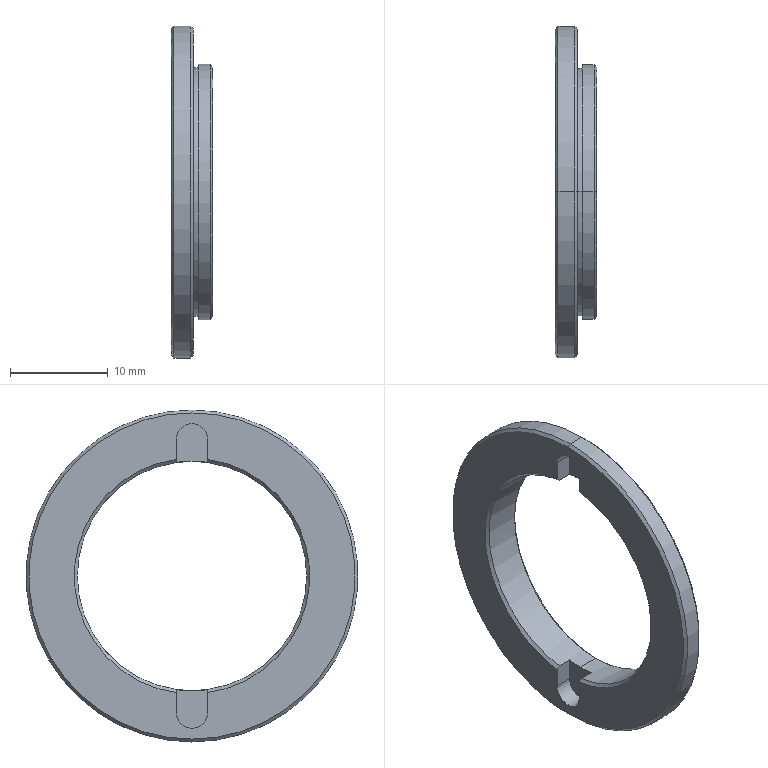Part | STEP file | CRM-1A-1-3-ZA.step-14.STEP.STEP-83.STEP | 1 solid | 31 faces | box 4.3 x 34 x 34 mm | volume 1225 mm3 | cylinder 11 | cone 10 | plane 10 | commonest cylinder face diameters 3.2 x3 23.5 x2 25.4 x2 26.2 x2 34 x2
STEP:
#1=CARTESIAN_POINT('',(1.8,0.,15.6));
#2=VERTEX_POINT('',#1);
#3=CARTESIAN_POINT('',(1.8,1.6,14.));
#4=VERTEX_POINT('',#3);
#5=CARTESIAN_POINT('',(1.8,0.,14.));
#6=DIRECTION('',(-1.,0.,0.));
#7=DIRECTION('',(0.,0.,-1.));
#8=AXIS2_PLACEMENT_3D('',#5,#6,#7);
#9=CIRCLE('',#8,1.6);
#10=EDGE_CURVE('',#2,#4,#9,.T.);
#11=ORIENTED_EDGE('',*,*,#10,.F.);
#12=CARTESIAN_POINT('',(0.,0.,15.6));
#13=VERTEX_POINT('',#12);
#14=CARTESIAN_POINT('',(1.8,0.,15.6));
#15=DIRECTION('',(-1.,0.,0.));
#16=VECTOR('',#15,1000.);
#17=LINE('',#14,#16);
#18=EDGE_CURVE('',#2,#13,#17,.T.);
#19=ORIENTED_EDGE('',*,*,#18,.T.);
#20=CARTESIAN_POINT('',(0.,1.6,14.));
#21=VERTEX_POINT('',#20);
#22=CARTESIAN_POINT('',(0.,0.,14.));
#23=DIRECTION('',(-1.,0.,0.));
#24=DIRECTION('',(0.,0.,-1.));
#25=AXIS2_PLACEMENT_3D('',#22,#23,#24);
#26=CIRCLE('',#25,1.6);
#27=EDGE_CURVE('',#13,#21,#26,.T.);
#28=ORIENTED_EDGE('',*,*,#27,.T.);
#29=CARTESIAN_POINT('',(1.8,1.6,14.));
#30=DIRECTION('',(-1.,0.,0.));
#31=VECTOR('',#30,1000.);
#32=LINE('',#29,#31);
#33=EDGE_CURVE('',#4,#21,#32,.T.);
#34=ORIENTED_EDGE('',*,*,#33,.F.);
#35=EDGE_LOOP('',(#11,#19,#28,#34));
#36=FACE_OUTER_BOUND('',#35,.T.);
#37=CARTESIAN_POINT('',(1.8,0.,14.));
#38=DIRECTION('',(-1.,0.,0.));
#39=DIRECTION('',(0.,0.,1.));
#40=AXIS2_PLACEMENT_3D('',#37,#38,#39);
#41=CYLINDRICAL_SURFACE('',#40,1.6);
#42=ADVANCED_FACE('',(#36),#41,.F.);
#43=CARTESIAN_POINT('',(4.3,0.,-12.8));
#44=VERTEX_POINT('',#43);
#45=CARTESIAN_POINT('',(4.3,0.,12.8));
#46=VERTEX_POINT('',#45);
#47=CARTESIAN_POINT('',(4.3,0.,0.));
#48=DIRECTION('',(1.,0.,0.));
#49=DIRECTION('',(0.,0.,1.));
#50=AXIS2_PLACEMENT_3D('',#47,#48,#49);
#51=CIRCLE('',#50,12.8);
#52=EDGE_CURVE('',#44,#46,#51,.T.);
#53=ORIENTED_EDGE('',*,*,#52,.F.);
#54=CARTESIAN_POINT('',(4.,0.,-13.1));
#55=VERTEX_POINT('',#54);
#56=CARTESIAN_POINT('',(4.,0.,-13.1));
#57=DIRECTION('',(-0.7071,0.,-0.7071));
#58=VECTOR('',#57,1000.);
#59=LINE('',#56,#58);
#60=EDGE_CURVE('',#44,#55,#59,.T.);
#61=ORIENTED_EDGE('',*,*,#60,.T.);
#62=CARTESIAN_POINT('',(4.,0.,13.1));
#63=VERTEX_POINT('',#62);
#64=CARTESIAN_POINT('',(4.,0.,0.));
#65=DIRECTION('',(-1.,0.,0.));
#66=DIRECTION('',(0.,0.,1.));
#67=AXIS2_PLACEMENT_3D('',#64,#65,#66);
#68=CIRCLE('',#67,13.1);
#69=EDGE_CURVE('',#63,#55,#68,.T.);
#70=ORIENTED_EDGE('',*,*,#69,.F.);
#71=CARTESIAN_POINT('',(4.,0.,13.1));
#72=DIRECTION('',(-0.7071,0.,0.7071));
#73=VECTOR('',#72,1000.);
#74=LINE('',#71,#73);
#75=EDGE_CURVE('',#46,#63,#74,.T.);
#76=ORIENTED_EDGE('',*,*,#75,.F.);
#77=EDGE_LOOP('',(#53,#61,#70,#76));
#78=FACE_OUTER_BOUND('',#77,.T.);
#79=CARTESIAN_POINT('',(4.,0.,0.));
#80=DIRECTION('',(-1.,0.,0.));
#81=DIRECTION('',(0.,0.,1.));
#82=AXIS2_PLACEMENT_3D('',#79,#80,#81);
#83=CONICAL_SURFACE('',#82,13.1,0.7854);
#84=ADVANCED_FACE('',(#78),#83,.T.);
#85=CARTESIAN_POINT('',(2.3,0.,-16.7));
#86=VERTEX_POINT('',#85);
#87=CARTESIAN_POINT('',(2.3,0.,16.7));
#88=VERTEX_POINT('',#87);
#89=CARTESIAN_POINT('',(2.3,0.,0.));
#90=DIRECTION('',(1.,0.,0.));
#91=DIRECTION('',(0.,0.,1.));
#92=AXIS2_PLACEMENT_3D('',#89,#90,#91);
#93=CIRCLE('',#92,16.7);
#94=EDGE_CURVE('',#86,#88,#93,.T.);
#95=ORIENTED_EDGE('',*,*,#94,.F.);
#96=CARTESIAN_POINT('',(2.,0.,-17.));
#97=VERTEX_POINT('',#96);
#98=CARTESIAN_POINT('',(2.,0.,-17.));
#99=DIRECTION('',(-0.7071,0.,-0.7071));
#100=VECTOR('',#99,1000.);
#101=LINE('',#98,#100);
#102=EDGE_CURVE('',#86,#97,#101,.T.);
#103=ORIENTED_EDGE('',*,*,#102,.T.);
#104=CARTESIAN_POINT('',(2.,0.,17.));
#105=VERTEX_POINT('',#104);
#106=CARTESIAN_POINT('',(2.,0.,0.));
#107=DIRECTION('',(-1.,0.,0.));
#108=DIRECTION('',(0.,0.,1.));
#109=AXIS2_PLACEMENT_3D('',#106,#107,#108);
#110=CIRCLE('',#109,17.);
#111=EDGE_CURVE('',#105,#97,#110,.T.);
#112=ORIENTED_EDGE('',*,*,#111,.F.);
#113=CARTESIAN_POINT('',(2.,0.,17.));
#114=DIRECTION('',(-0.7071,0.,0.7071));
#115=VECTOR('',#114,1000.);
#116=LINE('',#113,#115);
#117=EDGE_CURVE('',#88,#105,#116,.T.);
#118=ORIENTED_EDGE('',*,*,#117,.F.);
#119=EDGE_LOOP('',(#95,#103,#112,#118));
#120=FACE_OUTER_BOUND('',#119,.T.);
#121=CARTESIAN_POINT('',(2.,0.,0.));
#122=DIRECTION('',(-1.,0.,0.));
#123=DIRECTION('',(0.,0.,1.));
#124=AXIS2_PLACEMENT_3D('',#121,#122,#123);
#125=CONICAL_SURFACE('',#124,17.,0.7854);
#126=ADVANCED_FACE('',(#120),#125,.T.);
#127=CARTESIAN_POINT('',(0.,0.,16.7));
#128=VERTEX_POINT('',#127);
#129=CARTESIAN_POINT('',(0.,0.,-16.7));
#130=VERTEX_POINT('',#129);
#131=CARTESIAN_POINT('',(0.,0.,0.));
#132=DIRECTION('',(-1.,0.,0.));
#133=DIRECTION('',(0.,0.,-1.));
#134=AXIS2_PLACEMENT_3D('',#131,#132,#133);
#135=CIRCLE('',#134,16.7);
#136=EDGE_CURVE('',#128,#130,#135,.T.);
#137=ORIENTED_EDGE('',*,*,#136,.F.);
#138=CARTESIAN_POINT('',(0.3,0.,17.));
#139=VERTEX_POINT('',#138);
#140=CARTESIAN_POINT('',(0.,0.,16.7));
#141=DIRECTION('',(0.7071,0.,0.7071));
#142=VECTOR('',#141,1000.);
#143=LINE('',#140,#142);
#144=EDGE_CURVE('',#128,#139,#143,.T.);
#145=ORIENTED_EDGE('',*,*,#144,.T.);
#146=CARTESIAN_POINT('',(0.3,0.,-17.));
#147=VERTEX_POINT('',#146);
#148=CARTESIAN_POINT('',(0.3,0.,0.));
#149=DIRECTION('',(1.,0.,0.));
#150=DIRECTION('',(0.,0.,-1.));
#151=AXIS2_PLACEMENT_3D('',#148,#149,#150);
#152=CIRCLE('',#151,17.);
#153=EDGE_CURVE('',#147,#139,#152,.T.);
#154=ORIENTED_EDGE('',*,*,#153,.F.);
#155=CARTESIAN_POINT('',(0.,0.,-16.7));
#156=DIRECTION('',(0.7071,0.,-0.7071));
#157=VECTOR('',#156,1000.);
#158=LINE('',#155,#157);
#159=EDGE_CURVE('',#130,#147,#158,.T.);
#160=ORIENTED_EDGE('',*,*,#159,.F.);
#161=EDGE_LOOP('',(#137,#145,#154,#160));
#162=FACE_OUTER_BOUND('',#161,.T.);
#163=CARTESIAN_POINT('',(0.,0.,0.));
#164=DIRECTION('',(1.,0.,0.));
#165=DIRECTION('',(0.,0.,-1.));
#166=AXIS2_PLACEMENT_3D('',#163,#164,#165);
#167=CONICAL_SURFACE('',#166,16.7,0.7854);
#168=ADVANCED_FACE('',(#162),#167,.T.);
#169=CARTESIAN_POINT('',(4.,0.,11.75));
#170=VERTEX_POINT('',#169);
#171=CARTESIAN_POINT('',(4.,0.,-11.75));
#172=VERTEX_POINT('',#171);
#173=CARTESIAN_POINT('',(4.,0.,0.));
#174=DIRECTION('',(1.,0.,0.));
#175=DIRECTION('',(0.,0.,1.));
#176=AXIS2_PLACEMENT_3D('',#173,#174,#175);
#177=CIRCLE('',#176,11.75);
#178=EDGE_CURVE('',#170,#172,#177,.T.);
#179=ORIENTED_EDGE('',*,*,#178,.F.);
#180=CARTESIAN_POINT('',(4.3,0.,12.05));
#181=VERTEX_POINT('',#180);
#182=CARTESIAN_POINT('',(4.3,0.,12.05));
#183=DIRECTION('',(0.7071,0.,0.7071));
#184=VECTOR('',#183,1000.);
#185=LINE('',#182,#184);
#186=EDGE_CURVE('',#170,#181,#185,.T.);
#187=ORIENTED_EDGE('',*,*,#186,.T.);
#188=CARTESIAN_POINT('',(4.3,0.,-12.05));
#189=VERTEX_POINT('',#188);
#190=CARTESIAN_POINT('',(4.3,0.,0.));
#191=DIRECTION('',(-1.,0.,0.));
#192=DIRECTION('',(0.,0.,1.));
#193=AXIS2_PLACEMENT_3D('',#190,#191,#192);
#194=CIRCLE('',#193,12.05);
#195=EDGE_CURVE('',#189,#181,#194,.T.);
#196=ORIENTED_EDGE('',*,*,#195,.F.);
#197=CARTESIAN_POINT('',(4.3,0.,-12.05));
#198=DIRECTION('',(0.7071,0.,-0.7071));
#199=VECTOR('',#198,1000.);
#200=LINE('',#197,#199);
#201=EDGE_CURVE('',#172,#189,#200,.T.);
#202=ORIENTED_EDGE('',*,*,#201,.F.);
#203=EDGE_LOOP('',(#179,#187,#196,#202));
#204=FACE_OUTER_BOUND('',#203,.T.);
#205=CARTESIAN_POINT('',(4.3,0.,0.));
#206=DIRECTION('',(1.,0.,0.));
#207=DIRECTION('',(0.,0.,-1.));
#208=AXIS2_PLACEMENT_3D('',#205,#206,#207);
#209=CONICAL_SURFACE('',#208,12.05,0.7854);
#210=ADVANCED_FACE('',(#204),#209,.F.);
#211=ORIENTED_EDGE('',*,*,#178,.T.);
#212=CARTESIAN_POINT('',(1.8,0.,-11.75));
#213=VERTEX_POINT('',#212);
#214=CARTESIAN_POINT('',(0.,0.,-11.75));
#215=DIRECTION('',(-1.,0.,0.));
#216=VECTOR('',#215,1000.);
#217=LINE('',#214,#216);
#218=EDGE_CURVE('',#172,#213,#217,.T.);
#219=ORIENTED_EDGE('',*,*,#218,.T.);
#220=CARTESIAN_POINT('',(1.8,-1.6,-11.641));
#221=VERTEX_POINT('',#220);
#222=CARTESIAN_POINT('',(1.8,0.,0.));
#223=DIRECTION('',(1.,0.,0.));
#224=DIRECTION('',(0.,0.,1.));
#225=AXIS2_PLACEMENT_3D('',#222,#223,#224);
#226=CIRCLE('',#225,11.75);
#227=EDGE_CURVE('',#221,#213,#226,.T.);
#228=ORIENTED_EDGE('',*,*,#227,.F.);
#229=CARTESIAN_POINT('',(0.3,-1.6,-11.641));
#230=VERTEX_POINT('',#229);
#231=CARTESIAN_POINT('',(0.,-1.6,-11.641));
#232=DIRECTION('',(-1.,0.,0.));
#233=VECTOR('',#232,1000.);
#234=LINE('',#231,#233);
#235=EDGE_CURVE('',#221,#230,#234,.T.);
#236=ORIENTED_EDGE('',*,*,#235,.T.);
#237=CARTESIAN_POINT('',(0.3,-1.6,11.641));
#238=VERTEX_POINT('',#237);
#239=CARTESIAN_POINT('',(0.3,0.,0.));
#240=DIRECTION('',(-1.,0.,0.));
#241=DIRECTION('',(0.,0.,-1.));
#242=AXIS2_PLACEMENT_3D('',#239,#240,#241);
#243=CIRCLE('',#242,11.75);
#244=EDGE_CURVE('',#230,#238,#243,.T.);
#245=ORIENTED_EDGE('',*,*,#244,.T.);
#246=CARTESIAN_POINT('',(1.8,-1.6,11.641));
#247=VERTEX_POINT('',#246);
#248=CARTESIAN_POINT('',(0.,-1.6,11.641));
#249=DIRECTION('',(1.,0.,0.));
#250=VECTOR('',#249,1000.);
#251=LINE('',#248,#250);
#252=EDGE_CURVE('',#238,#247,#251,.T.);
#253=ORIENTED_EDGE('',*,*,#252,.T.);
#254=CARTESIAN_POINT('',(1.8,0.,11.75));
#255=VERTEX_POINT('',#254);
#256=CARTESIAN_POINT('',(1.8,0.,0.));
#257=DIRECTION('',(1.,0.,0.));
#258=DIRECTION('',(0.,0.,1.));
#259=AXIS2_PLACEMENT_3D('',#256,#257,#258);
#260=CIRCLE('',#259,11.75);
#261=EDGE_CURVE('',#255,#247,#260,.T.);
#262=ORIENTED_EDGE('',*,*,#261,.F.);
#263=CARTESIAN_POINT('',(0.,0.,11.75));
#264=DIRECTION('',(-1.,0.,0.));
#265=VECTOR('',#264,1000.);
#266=LINE('',#263,#265);
#267=EDGE_CURVE('',#170,#255,#266,.T.);
#268=ORIENTED_EDGE('',*,*,#267,.F.);
#269=EDGE_LOOP('',(#211,#219,#228,#236,#245,#253,#262,#268));
#270=FACE_OUTER_BOUND('',#269,.T.);
#271=CARTESIAN_POINT('',(0.,0.,0.));
#272=DIRECTION('',(-1.,0.,0.));
#273=DIRECTION('',(0.,0.,1.));
#274=AXIS2_PLACEMENT_3D('',#271,#272,#273);
#275=CYLINDRICAL_SURFACE('',#274,11.75);
#276=ADVANCED_FACE('',(#270),#275,.F.);
#277=ORIENTED_EDGE('',*,*,#69,.T.);
#278=CARTESIAN_POINT('',(2.8,0.,-13.1));
#279=VERTEX_POINT('',#278);
#280=CARTESIAN_POINT('',(0.,0.,-13.1));
#281=DIRECTION('',(-1.,0.,0.));
#282=VECTOR('',#281,1000.);
#283=LINE('',#280,#282);
#284=EDGE_CURVE('',#55,#279,#283,.T.);
#285=ORIENTED_EDGE('',*,*,#284,.T.);
#286=CARTESIAN_POINT('',(2.8,0.,13.1));
#287=VERTEX_POINT('',#286);
#288=CARTESIAN_POINT('',(2.8,0.,0.));
#289=DIRECTION('',(-1.,0.,0.));
#290=DIRECTION('',(0.,0.,1.));
#291=AXIS2_PLACEMENT_3D('',#288,#289,#290);
#292=CIRCLE('',#291,13.1);
#293=EDGE_CURVE('',#287,#279,#292,.T.);
#294=ORIENTED_EDGE('',*,*,#293,.F.);
#295=CARTESIAN_POINT('',(0.,0.,13.1));
#296=DIRECTION('',(-1.,0.,0.));
#297=VECTOR('',#296,1000.);
#298=LINE('',#295,#297);
#299=EDGE_CURVE('',#63,#287,#298,.T.);
#300=ORIENTED_EDGE('',*,*,#299,.F.);
#301=EDGE_LOOP('',(#277,#285,#294,#300));
#302=FACE_OUTER_BOUND('',#301,.T.);
#303=CARTESIAN_POINT('',(0.,0.,0.));
#304=DIRECTION('',(-1.,0.,0.));
#305=DIRECTION('',(0.,0.,1.));
#306=AXIS2_PLACEMENT_3D('',#303,#304,#305);
#307=CYLINDRICAL_SURFACE('',#306,13.1);
#308=ADVANCED_FACE('',(#302),#307,.T.);
#309=CARTESIAN_POINT('',(2.8,0.,12.7));
#310=VERTEX_POINT('',#309);
#311=CARTESIAN_POINT('',(2.8,0.,-12.7));
#312=VERTEX_POINT('',#311);
#313=CARTESIAN_POINT('',(2.8,0.,0.));
#314=DIRECTION('',(-1.,0.,0.));
#315=DIRECTION('',(0.,0.,1.));
#316=AXIS2_PLACEMENT_3D('',#313,#314,#315);
#317=CIRCLE('',#316,12.7);
#318=EDGE_CURVE('',#310,#312,#317,.T.);
#319=ORIENTED_EDGE('',*,*,#318,.T.);
#320=CARTESIAN_POINT('',(2.3,0.,-12.7));
#321=VERTEX_POINT('',#320);
#322=CARTESIAN_POINT('',(0.,0.,-12.7));
#323=DIRECTION('',(-1.,0.,0.));
#324=VECTOR('',#323,1000.);
#325=LINE('',#322,#324);
#326=EDGE_CURVE('',#312,#321,#325,.T.);
#327=ORIENTED_EDGE('',*,*,#326,.T.);
#328=CARTESIAN_POINT('',(2.3,0.,12.7));
#329=VERTEX_POINT('',#328);
#330=CARTESIAN_POINT('',(2.3,0.,0.));
#331=DIRECTION('',(-1.,0.,0.));
#332=DIRECTION('',(0.,0.,1.));
#333=AXIS2_PLACEMENT_3D('',#330,#331,#332);
#334=CIRCLE('',#333,12.7);
#335=EDGE_CURVE('',#329,#321,#334,.T.);
#336=ORIENTED_EDGE('',*,*,#335,.F.);
#337=CARTESIAN_POINT('',(0.,0.,12.7));
#338=DIRECTION('',(-1.,0.,0.));
#339=VECTOR('',#338,1000.);
#340=LINE('',#337,#339);
#341=EDGE_CURVE('',#310,#329,#340,.T.);
#342=ORIENTED_EDGE('',*,*,#341,.F.);
#343=EDGE_LOOP('',(#319,#327,#336,#342));
#344=FACE_OUTER_BOUND('',#343,.T.);
#345=CARTESIAN_POINT('',(0.,0.,0.));
#346=DIRECTION('',(-1.,0.,0.));
#347=DIRECTION('',(0.,0.,1.));
#348=AXIS2_PLACEMENT_3D('',#345,#346,#347);
#349=CYLINDRICAL_SURFACE('',#348,12.7);
#350=ADVANCED_FACE('',(#344),#349,.T.);
#351=ORIENTED_EDGE('',*,*,#111,.T.);
#352=CARTESIAN_POINT('',(0.,0.,-17.));
#353=DIRECTION('',(-1.,0.,0.));
#354=VECTOR('',#353,1000.);
#355=LINE('',#352,#354);
#356=EDGE_CURVE('',#97,#147,#355,.T.);
#357=ORIENTED_EDGE('',*,*,#356,.T.);
#358=ORIENTED_EDGE('',*,*,#153,.T.);
#359=CARTESIAN_POINT('',(0.,0.,17.));
#360=DIRECTION('',(-1.,0.,0.));
#361=VECTOR('',#360,1000.);
#362=LINE('',#359,#361);
#363=EDGE_CURVE('',#105,#139,#362,.T.);
#364=ORIENTED_EDGE('',*,*,#363,.F.);
#365=EDGE_LOOP('',(#351,#357,#358,#364));
#366=FACE_OUTER_BOUND('',#365,.T.);
#367=CARTESIAN_POINT('',(0.,0.,0.));
#368=DIRECTION('',(-1.,0.,0.));
#369=DIRECTION('',(0.,0.,1.));
#370=AXIS2_PLACEMENT_3D('',#367,#368,#369);
#371=CYLINDRICAL_SURFACE('',#370,17.);
#372=ADVANCED_FACE('',(#366),#371,.T.);
#373=CARTESIAN_POINT('',(0.,1.6,11.943));
#374=VERTEX_POINT('',#373);
#375=CARTESIAN_POINT('',(0.3,1.6,11.641));
#376=VERTEX_POINT('',#375);
#377=CARTESIAN_POINT('',(0.,1.6,11.943));
#378=CARTESIAN_POINT('',(0.1,1.6,11.842));
#379=CARTESIAN_POINT('',(0.2,1.6,11.741));
#380=CARTESIAN_POINT('',(0.3,1.6,11.641));
#381=B_SPLINE_CURVE_WITH_KNOTS('',3,(#377,#378,#379,#380),.UNSPECIFIED.,.F.,.F.,(4,4),(0.02049,0.02092),.UNSPECIFIED.);
#382=EDGE_CURVE('',#374,#376,#381,.T.);
#383=ORIENTED_EDGE('',*,*,#382,.F.);
#384=CARTESIAN_POINT('',(0.,1.6,-11.943));
#385=VERTEX_POINT('',#384);
#386=CARTESIAN_POINT('',(0.,0.,0.));
#387=DIRECTION('',(1.,0.,0.));
#388=DIRECTION('',(0.,0.,-1.));
#389=AXIS2_PLACEMENT_3D('',#386,#387,#388);
#390=CIRCLE('',#389,12.05);
#391=EDGE_CURVE('',#385,#374,#390,.T.);
#392=ORIENTED_EDGE('',*,*,#391,.F.);
#393=CARTESIAN_POINT('',(0.3,1.6,-11.641));
#394=VERTEX_POINT('',#393);
#395=CARTESIAN_POINT('',(0.3,1.6,-11.641));
#396=CARTESIAN_POINT('',(0.2,1.6,-11.741));
#397=CARTESIAN_POINT('',(0.1,1.6,-11.842));
#398=CARTESIAN_POINT('',(0.,1.6,-11.943));
#399=B_SPLINE_CURVE_WITH_KNOTS('',3,(#395,#396,#397,#398),.UNSPECIFIED.,.F.,.F.,(4,4),(0.05212,0.05255),.UNSPECIFIED.);
#400=EDGE_CURVE('',#394,#385,#399,.T.);
#401=ORIENTED_EDGE('',*,*,#400,.F.);
#402=CARTESIAN_POINT('',(0.3,0.,0.));
#403=DIRECTION('',(-1.,0.,0.));
#404=DIRECTION('',(0.,0.,-1.));
#405=AXIS2_PLACEMENT_3D('',#402,#403,#404);
#406=CIRCLE('',#405,11.75);
#407=EDGE_CURVE('',#376,#394,#406,.T.);
#408=ORIENTED_EDGE('',*,*,#407,.F.);
#409=EDGE_LOOP('',(#383,#392,#401,#408));
#410=FACE_OUTER_BOUND('',#409,.T.);
#411=CARTESIAN_POINT('',(0.3,0.,0.));
#412=DIRECTION('',(-1.,0.,0.));
#413=DIRECTION('',(0.,0.,1.));
#414=AXIS2_PLACEMENT_3D('',#411,#412,#413);
#415=CONICAL_SURFACE('',#414,11.75,0.7854);
#416=ADVANCED_FACE('',(#410),#415,.F.);
#417=ORIENTED_EDGE('',*,*,#356,.F.);
#418=CARTESIAN_POINT('',(2.,0.,0.));
#419=DIRECTION('',(-1.,0.,0.));
#420=DIRECTION('',(0.,0.,1.));
#421=AXIS2_PLACEMENT_3D('',#418,#419,#420);
#422=CIRCLE('',#421,17.);
#423=EDGE_CURVE('',#97,#105,#422,.T.);
#424=ORIENTED_EDGE('',*,*,#423,.T.);
#425=ORIENTED_EDGE('',*,*,#363,.T.);
#426=CARTESIAN_POINT('',(0.3,0.,0.));
#427=DIRECTION('',(1.,0.,0.));
#428=DIRECTION('',(0.,0.,-1.));
#429=AXIS2_PLACEMENT_3D('',#426,#427,#428);
#430=CIRCLE('',#429,17.);
#431=EDGE_CURVE('',#139,#147,#430,.T.);
#432=ORIENTED_EDGE('',*,*,#431,.T.);
#433=EDGE_LOOP('',(#417,#424,#425,#432));
#434=FACE_OUTER_BOUND('',#433,.T.);
#435=CARTESIAN_POINT('',(0.,0.,0.));
#436=DIRECTION('',(-1.,0.,0.));
#437=DIRECTION('',(0.,0.,1.));
#438=AXIS2_PLACEMENT_3D('',#435,#436,#437);
#439=CYLINDRICAL_SURFACE('',#438,17.);
#440=ADVANCED_FACE('',(#434),#439,.T.);
#441=ORIENTED_EDGE('',*,*,#335,.T.);
#442=CARTESIAN_POINT('',(2.3,0.,0.));
#443=DIRECTION('',(-1.,0.,0.));
#444=DIRECTION('',(0.,0.,1.));
#445=AXIS2_PLACEMENT_3D('',#442,#443,#444);
#446=CIRCLE('',#445,12.7);
#447=EDGE_CURVE('',#321,#329,#446,.T.);
#448=ORIENTED_EDGE('',*,*,#447,.T.);
#449=EDGE_LOOP('',(#441,#448));
#450=FACE_BOUND('',#449,.T.);
#451=CARTESIAN_POINT('',(2.3,0.,0.));
#452=DIRECTION('',(1.,0.,0.));
#453=DIRECTION('',(0.,0.,1.));
#454=AXIS2_PLACEMENT_3D('',#451,#452,#453);
#455=CIRCLE('',#454,16.7);
#456=EDGE_CURVE('',#88,#86,#455,.T.);
#457=ORIENTED_EDGE('',*,*,#456,.T.);
#458=ORIENTED_EDGE('',*,*,#94,.T.);
#459=EDGE_LOOP('',(#457,#458));
#460=FACE_OUTER_BOUND('',#459,.T.);
#461=CARTESIAN_POINT('',(2.3,12.7,0.));
#462=DIRECTION('',(-1.,0.,0.));
#463=DIRECTION('',(0.,0.,1.));
#464=AXIS2_PLACEMENT_3D('',#461,#462,#463);
#465=PLANE('',#464);
#466=ADVANCED_FACE('',(#450,#460),#465,.F.);
#467=ORIENTED_EDGE('',*,*,#326,.F.);
#468=CARTESIAN_POINT('',(2.8,0.,0.));
#469=DIRECTION('',(-1.,0.,0.));
#470=DIRECTION('',(0.,0.,1.));
#471=AXIS2_PLACEMENT_3D('',#468,#469,#470);
#472=CIRCLE('',#471,12.7);
#473=EDGE_CURVE('',#312,#310,#472,.T.);
#474=ORIENTED_EDGE('',*,*,#473,.T.);
#475=ORIENTED_EDGE('',*,*,#341,.T.);
#476=ORIENTED_EDGE('',*,*,#447,.F.);
#477=EDGE_LOOP('',(#467,#474,#475,#476));
#478=FACE_OUTER_BOUND('',#477,.T.);
#479=CARTESIAN_POINT('',(0.,0.,0.));
#480=DIRECTION('',(-1.,0.,0.));
#481=DIRECTION('',(0.,0.,1.));
#482=AXIS2_PLACEMENT_3D('',#479,#480,#481);
#483=CYLINDRICAL_SURFACE('',#482,12.7);
#484=ADVANCED_FACE('',(#478),#483,.T.);
#485=ORIENTED_EDGE('',*,*,#318,.F.);
#486=ORIENTED_EDGE('',*,*,#473,.F.);
#487=EDGE_LOOP('',(#485,#486));
#488=FACE_BOUND('',#487,.T.);
#489=ORIENTED_EDGE('',*,*,#293,.T.);
#490=CARTESIAN_POINT('',(2.8,0.,0.));
#491=DIRECTION('',(-1.,0.,0.));
#492=DIRECTION('',(0.,0.,1.));
#493=AXIS2_PLACEMENT_3D('',#490,#491,#492);
#494=CIRCLE('',#493,13.1);
#495=EDGE_CURVE('',#279,#287,#494,.T.);
#496=ORIENTED_EDGE('',*,*,#495,.T.);
#497=EDGE_LOOP('',(#489,#496));
#498=FACE_OUTER_BOUND('',#497,.T.);
#499=CARTESIAN_POINT('',(2.8,13.1,0.));
#500=DIRECTION('',(1.,0.,0.));
#501=DIRECTION('',(0.,1.,0.));
#502=AXIS2_PLACEMENT_3D('',#499,#500,#501);
#503=PLANE('',#502);
#504=ADVANCED_FACE('',(#488,#498),#503,.F.);
#505=ORIENTED_EDGE('',*,*,#284,.F.);
#506=CARTESIAN_POINT('',(4.,0.,0.));
#507=DIRECTION('',(-1.,0.,0.));
#508=DIRECTION('',(0.,0.,1.));
#509=AXIS2_PLACEMENT_3D('',#506,#507,#508);
#510=CIRCLE('',#509,13.1);
#511=EDGE_CURVE('',#55,#63,#510,.T.);
#512=ORIENTED_EDGE('',*,*,#511,.T.);
#513=ORIENTED_EDGE('',*,*,#299,.T.);
#514=ORIENTED_EDGE('',*,*,#495,.F.);
#515=EDGE_LOOP('',(#505,#512,#513,#514));
#516=FACE_OUTER_BOUND('',#515,.T.);
#517=CARTESIAN_POINT('',(0.,0.,0.));
#518=DIRECTION('',(-1.,0.,0.));
#519=DIRECTION('',(0.,0.,1.));
#520=AXIS2_PLACEMENT_3D('',#517,#518,#519);
#521=CYLINDRICAL_SURFACE('',#520,13.1);
#522=ADVANCED_FACE('',(#516),#521,.T.);
#523=ORIENTED_EDGE('',*,*,#195,.T.);
#524=CARTESIAN_POINT('',(4.3,0.,0.));
#525=DIRECTION('',(-1.,0.,0.));
#526=DIRECTION('',(0.,0.,1.));
#527=AXIS2_PLACEMENT_3D('',#524,#525,#526);
#528=CIRCLE('',#527,12.05);
#529=EDGE_CURVE('',#181,#189,#528,.T.);
#530=ORIENTED_EDGE('',*,*,#529,.T.);
#531=EDGE_LOOP('',(#523,#530));
#532=FACE_BOUND('',#531,.T.);
#533=CARTESIAN_POINT('',(4.3,0.,0.));
#534=DIRECTION('',(1.,0.,0.));
#535=DIRECTION('',(0.,0.,1.));
#536=AXIS2_PLACEMENT_3D('',#533,#534,#535);
#537=CIRCLE('',#536,12.8);
#538=EDGE_CURVE('',#46,#44,#537,.T.);
#539=ORIENTED_EDGE('',*,*,#538,.T.);
#540=ORIENTED_EDGE('',*,*,#52,.T.);
#541=EDGE_LOOP('',(#539,#540));
#542=FACE_OUTER_BOUND('',#541,.T.);
#543=CARTESIAN_POINT('',(4.3,13.1,0.));
#544=DIRECTION('',(-1.,0.,0.));
#545=DIRECTION('',(0.,0.,1.));
#546=AXIS2_PLACEMENT_3D('',#543,#544,#545);
#547=PLANE('',#546);
#548=ADVANCED_FACE('',(#532,#542),#547,.F.);
#549=ORIENTED_EDGE('',*,*,#218,.F.);
#550=CARTESIAN_POINT('',(4.,0.,0.));
#551=DIRECTION('',(1.,0.,0.));
#552=DIRECTION('',(0.,0.,1.));
#553=AXIS2_PLACEMENT_3D('',#550,#551,#552);
#554=CIRCLE('',#553,11.75);
#555=EDGE_CURVE('',#172,#170,#554,.T.);
#556=ORIENTED_EDGE('',*,*,#555,.T.);
#557=ORIENTED_EDGE('',*,*,#267,.T.);
#558=CARTESIAN_POINT('',(1.8,1.6,11.641));
#559=VERTEX_POINT('',#558);
#560=CARTESIAN_POINT('',(1.8,0.,0.));
#561=DIRECTION('',(1.,0.,0.));
#562=DIRECTION('',(0.,0.,1.));
#563=AXIS2_PLACEMENT_3D('',#560,#561,#562);
#564=CIRCLE('',#563,11.75);
#565=EDGE_CURVE('',#559,#255,#564,.T.);
#566=ORIENTED_EDGE('',*,*,#565,.F.);
#567=CARTESIAN_POINT('',(0.,1.6,11.641));
#568=DIRECTION('',(-1.,0.,0.));
#569=VECTOR('',#568,1000.);
#570=LINE('',#567,#569);
#571=EDGE_CURVE('',#559,#376,#570,.T.);
#572=ORIENTED_EDGE('',*,*,#571,.T.);
#573=ORIENTED_EDGE('',*,*,#407,.T.);
#574=CARTESIAN_POINT('',(1.8,1.6,-11.641));
#575=VERTEX_POINT('',#574);
#576=CARTESIAN_POINT('',(0.,1.6,-11.641));
#577=DIRECTION('',(1.,0.,0.));
#578=VECTOR('',#577,1000.);
#579=LINE('',#576,#578);
#580=EDGE_CURVE('',#394,#575,#579,.T.);
#581=ORIENTED_EDGE('',*,*,#580,.T.);
#582=CARTESIAN_POINT('',(1.8,0.,0.));
#583=DIRECTION('',(1.,0.,0.));
#584=DIRECTION('',(0.,0.,1.));
#585=AXIS2_PLACEMENT_3D('',#582,#583,#584);
#586=CIRCLE('',#585,11.75);
#587=EDGE_CURVE('',#213,#575,#586,.T.);
#588=ORIENTED_EDGE('',*,*,#587,.F.);
#589=EDGE_LOOP('',(#549,#556,#557,#566,#572,#573,#581,#588));
#590=FACE_OUTER_BOUND('',#589,.T.);
#591=CARTESIAN_POINT('',(0.,0.,0.));
#592=DIRECTION('',(-1.,0.,0.));
#593=DIRECTION('',(0.,0.,1.));
#594=AXIS2_PLACEMENT_3D('',#591,#592,#593);
#595=CYLINDRICAL_SURFACE('',#594,11.75);
#596=ADVANCED_FACE('',(#590),#595,.F.);
#597=ORIENTED_EDGE('',*,*,#391,.T.);
#598=CARTESIAN_POINT('',(0.,1.6,0.));
#599=DIRECTION('',(0.,0.,-1.));
#600=VECTOR('',#599,1000.);
#601=LINE('',#598,#600);
#602=EDGE_CURVE('',#21,#374,#601,.T.);
#603=ORIENTED_EDGE('',*,*,#602,.F.);
#604=ORIENTED_EDGE('',*,*,#27,.F.);
#605=CARTESIAN_POINT('',(0.,-1.6,14.));
#606=VERTEX_POINT('',#605);
#607=CARTESIAN_POINT('',(0.,0.,14.));
#608=DIRECTION('',(-1.,0.,0.));
#609=DIRECTION('',(0.,0.,-1.));
#610=AXIS2_PLACEMENT_3D('',#607,#608,#609);
#611=CIRCLE('',#610,1.6);
#612=EDGE_CURVE('',#606,#13,#611,.T.);
#613=ORIENTED_EDGE('',*,*,#612,.F.);
#614=CARTESIAN_POINT('',(0.,-1.6,11.943));
#615=VERTEX_POINT('',#614);
#616=CARTESIAN_POINT('',(0.,-1.6,0.));
#617=DIRECTION('',(0.,0.,1.));
#618=VECTOR('',#617,1000.);
#619=LINE('',#616,#618);
#620=EDGE_CURVE('',#615,#606,#619,.T.);
#621=ORIENTED_EDGE('',*,*,#620,.F.);
#622=CARTESIAN_POINT('',(0.,-1.6,-11.943));
#623=VERTEX_POINT('',#622);
#624=CARTESIAN_POINT('',(0.,0.,0.));
#625=DIRECTION('',(1.,0.,0.));
#626=DIRECTION('',(0.,0.,-1.));
#627=AXIS2_PLACEMENT_3D('',#624,#625,#626);
#628=CIRCLE('',#627,12.05);
#629=EDGE_CURVE('',#615,#623,#628,.T.);
#630=ORIENTED_EDGE('',*,*,#629,.T.);
#631=CARTESIAN_POINT('',(0.,-1.6,-14.));
#632=VERTEX_POINT('',#631);
#633=CARTESIAN_POINT('',(0.,-1.6,0.));
#634=DIRECTION('',(0.,0.,1.));
#635=VECTOR('',#634,1000.);
#636=LINE('',#633,#635);
#637=EDGE_CURVE('',#632,#623,#636,.T.);
#638=ORIENTED_EDGE('',*,*,#637,.F.);
#639=CARTESIAN_POINT('',(0.,1.6,-14.));
#640=VERTEX_POINT('',#639);
#641=CARTESIAN_POINT('',(0.,0.,-14.));
#642=DIRECTION('',(-1.,0.,0.));
#643=DIRECTION('',(0.,0.,1.));
#644=AXIS2_PLACEMENT_3D('',#641,#642,#643);
#645=CIRCLE('',#644,1.6);
#646=EDGE_CURVE('',#640,#632,#645,.T.);
#647=ORIENTED_EDGE('',*,*,#646,.F.);
#648=CARTESIAN_POINT('',(0.,1.6,0.));
#649=DIRECTION('',(0.,0.,-1.));
#650=VECTOR('',#649,1000.);
#651=LINE('',#648,#650);
#652=EDGE_CURVE('',#385,#640,#651,.T.);
#653=ORIENTED_EDGE('',*,*,#652,.F.);
#654=EDGE_LOOP('',(#597,#603,#604,#613,#621,#630,#638,#647,#653));
#655=FACE_BOUND('',#654,.T.);
#656=CARTESIAN_POINT('',(0.,0.,0.));
#657=DIRECTION('',(-1.,0.,0.));
#658=DIRECTION('',(0.,0.,-1.));
#659=AXIS2_PLACEMENT_3D('',#656,#657,#658);
#660=CIRCLE('',#659,16.7);
#661=EDGE_CURVE('',#130,#128,#660,.T.);
#662=ORIENTED_EDGE('',*,*,#661,.T.);
#663=ORIENTED_EDGE('',*,*,#136,.T.);
#664=EDGE_LOOP('',(#662,#663));
#665=FACE_OUTER_BOUND('',#664,.T.);
#666=CARTESIAN_POINT('',(0.,11.75,0.));
#667=DIRECTION('',(1.,0.,0.));
#668=DIRECTION('',(0.,1.,0.));
#669=AXIS2_PLACEMENT_3D('',#666,#667,#668);
#670=PLANE('',#669);
#671=ADVANCED_FACE('',(#655,#665),#670,.F.);
#672=CARTESIAN_POINT('',(0.,-1.6,-11.943));
#673=CARTESIAN_POINT('',(0.1,-1.6,-11.842));
#674=CARTESIAN_POINT('',(0.2,-1.6,-11.741));
#675=CARTESIAN_POINT('',(0.3,-1.6,-11.641));
#676=B_SPLINE_CURVE_WITH_KNOTS('',3,(#672,#673,#674,#675),.UNSPECIFIED.,.F.,.F.,(4,4),(0.02049,0.02092),.UNSPECIFIED.);
#677=EDGE_CURVE('',#623,#230,#676,.T.);
#678=ORIENTED_EDGE('',*,*,#677,.F.);
#679=ORIENTED_EDGE('',*,*,#629,.F.);
#680=CARTESIAN_POINT('',(0.3,-1.6,11.641));
#681=CARTESIAN_POINT('',(0.2,-1.6,11.741));
#682=CARTESIAN_POINT('',(0.1,-1.6,11.842));
#683=CARTESIAN_POINT('',(0.,-1.6,11.943));
#684=B_SPLINE_CURVE_WITH_KNOTS('',3,(#680,#681,#682,#683),.UNSPECIFIED.,.F.,.F.,(4,4),(0.05212,0.05255),.UNSPECIFIED.);
#685=EDGE_CURVE('',#238,#615,#684,.T.);
#686=ORIENTED_EDGE('',*,*,#685,.F.);
#687=ORIENTED_EDGE('',*,*,#244,.F.);
#688=EDGE_LOOP('',(#678,#679,#686,#687));
#689=FACE_OUTER_BOUND('',#688,.T.);
#690=CARTESIAN_POINT('',(0.3,0.,0.));
#691=DIRECTION('',(-1.,0.,0.));
#692=DIRECTION('',(0.,0.,1.));
#693=AXIS2_PLACEMENT_3D('',#690,#691,#692);
#694=CONICAL_SURFACE('',#693,11.75,0.7854);
#695=ADVANCED_FACE('',(#689),#694,.F.);
#696=ORIENTED_EDGE('',*,*,#186,.F.);
#697=ORIENTED_EDGE('',*,*,#555,.F.);
#698=ORIENTED_EDGE('',*,*,#201,.T.);
#699=ORIENTED_EDGE('',*,*,#529,.F.);
#700=EDGE_LOOP('',(#696,#697,#698,#699));
#701=FACE_OUTER_BOUND('',#700,.T.);
#702=CARTESIAN_POINT('',(4.3,0.,0.));
#703=DIRECTION('',(1.,0.,0.));
#704=DIRECTION('',(0.,0.,-1.));
#705=AXIS2_PLACEMENT_3D('',#702,#703,#704);
#706=CONICAL_SURFACE('',#705,12.05,0.7854);
#707=ADVANCED_FACE('',(#701),#706,.F.);
#708=ORIENTED_EDGE('',*,*,#144,.F.);
#709=ORIENTED_EDGE('',*,*,#661,.F.);
#710=ORIENTED_EDGE('',*,*,#159,.T.);
#711=ORIENTED_EDGE('',*,*,#431,.F.);
#712=EDGE_LOOP('',(#708,#709,#710,#711));
#713=FACE_OUTER_BOUND('',#712,.T.);
#714=CARTESIAN_POINT('',(0.,0.,0.));
#715=DIRECTION('',(1.,0.,0.));
#716=DIRECTION('',(0.,0.,-1.));
#717=AXIS2_PLACEMENT_3D('',#714,#715,#716);
#718=CONICAL_SURFACE('',#717,16.7,0.7854);
#719=ADVANCED_FACE('',(#713),#718,.T.);
#720=ORIENTED_EDGE('',*,*,#102,.F.);
#721=ORIENTED_EDGE('',*,*,#456,.F.);
#722=ORIENTED_EDGE('',*,*,#117,.T.);
#723=ORIENTED_EDGE('',*,*,#423,.F.);
#724=EDGE_LOOP('',(#720,#721,#722,#723));
#725=FACE_OUTER_BOUND('',#724,.T.);
#726=CARTESIAN_POINT('',(2.,0.,0.));
#727=DIRECTION('',(-1.,0.,0.));
#728=DIRECTION('',(0.,0.,1.));
#729=AXIS2_PLACEMENT_3D('',#726,#727,#728);
#730=CONICAL_SURFACE('',#729,17.,0.7854);
#731=ADVANCED_FACE('',(#725),#730,.T.);
#732=ORIENTED_EDGE('',*,*,#60,.F.);
#733=ORIENTED_EDGE('',*,*,#538,.F.);
#734=ORIENTED_EDGE('',*,*,#75,.T.);
#735=ORIENTED_EDGE('',*,*,#511,.F.);
#736=EDGE_LOOP('',(#732,#733,#734,#735));
#737=FACE_OUTER_BOUND('',#736,.T.);
#738=CARTESIAN_POINT('',(4.,0.,0.));
#739=DIRECTION('',(-1.,0.,0.));
#740=DIRECTION('',(0.,0.,1.));
#741=AXIS2_PLACEMENT_3D('',#738,#739,#740);
#742=CONICAL_SURFACE('',#741,13.1,0.7854);
#743=ADVANCED_FACE('',(#737),#742,.T.);
#744=CARTESIAN_POINT('',(1.8,1.6,0.));
#745=DIRECTION('',(0.,0.,-1.));
#746=VECTOR('',#745,1000.);
#747=LINE('',#744,#746);
#748=EDGE_CURVE('',#4,#559,#747,.T.);
#749=ORIENTED_EDGE('',*,*,#748,.F.);
#750=ORIENTED_EDGE('',*,*,#33,.T.);
#751=ORIENTED_EDGE('',*,*,#602,.T.);
#752=ORIENTED_EDGE('',*,*,#382,.T.);
#753=ORIENTED_EDGE('',*,*,#571,.F.);
#754=EDGE_LOOP('',(#749,#750,#751,#752,#753));
#755=FACE_OUTER_BOUND('',#754,.T.);
#756=CARTESIAN_POINT('',(1.8,1.6,0.));
#757=DIRECTION('',(0.,1.,0.));
#758=DIRECTION('',(1.,0.,0.));
#759=AXIS2_PLACEMENT_3D('',#756,#757,#758);
#760=PLANE('',#759);
#761=ADVANCED_FACE('',(#755),#760,.F.);
#762=ORIENTED_EDGE('',*,*,#685,.T.);
#763=ORIENTED_EDGE('',*,*,#620,.T.);
#764=CARTESIAN_POINT('',(1.8,-1.6,14.));
#765=VERTEX_POINT('',#764);
#766=CARTESIAN_POINT('',(1.8,-1.6,14.));
#767=DIRECTION('',(-1.,0.,0.));
#768=VECTOR('',#767,1000.);
#769=LINE('',#766,#768);
#770=EDGE_CURVE('',#765,#606,#769,.T.);
#771=ORIENTED_EDGE('',*,*,#770,.F.);
#772=CARTESIAN_POINT('',(1.8,-1.6,0.));
#773=DIRECTION('',(0.,0.,1.));
#774=VECTOR('',#773,1000.);
#775=LINE('',#772,#774);
#776=EDGE_CURVE('',#247,#765,#775,.T.);
#777=ORIENTED_EDGE('',*,*,#776,.F.);
#778=ORIENTED_EDGE('',*,*,#252,.F.);
#779=EDGE_LOOP('',(#762,#763,#771,#777,#778));
#780=FACE_OUTER_BOUND('',#779,.T.);
#781=CARTESIAN_POINT('',(1.8,-1.6,0.));
#782=DIRECTION('',(0.,-1.,0.));
#783=DIRECTION('',(0.,0.,-1.));
#784=AXIS2_PLACEMENT_3D('',#781,#782,#783);
#785=PLANE('',#784);
#786=ADVANCED_FACE('',(#780),#785,.F.);
#787=ORIENTED_EDGE('',*,*,#18,.F.);
#788=CARTESIAN_POINT('',(1.8,0.,14.));
#789=DIRECTION('',(-1.,0.,0.));
#790=DIRECTION('',(0.,0.,-1.));
#791=AXIS2_PLACEMENT_3D('',#788,#789,#790);
#792=CIRCLE('',#791,1.6);
#793=EDGE_CURVE('',#765,#2,#792,.T.);
#794=ORIENTED_EDGE('',*,*,#793,.F.);
#795=ORIENTED_EDGE('',*,*,#770,.T.);
#796=ORIENTED_EDGE('',*,*,#612,.T.);
#797=EDGE_LOOP('',(#787,#794,#795,#796));
#798=FACE_OUTER_BOUND('',#797,.T.);
#799=CARTESIAN_POINT('',(1.8,0.,14.));
#800=DIRECTION('',(-1.,0.,0.));
#801=DIRECTION('',(0.,0.,1.));
#802=AXIS2_PLACEMENT_3D('',#799,#800,#801);
#803=CYLINDRICAL_SURFACE('',#802,1.6);
#804=ADVANCED_FACE('',(#798),#803,.F.);
#805=ORIENTED_EDGE('',*,*,#565,.T.);
#806=ORIENTED_EDGE('',*,*,#261,.T.);
#807=ORIENTED_EDGE('',*,*,#776,.T.);
#808=ORIENTED_EDGE('',*,*,#793,.T.);
#809=ORIENTED_EDGE('',*,*,#10,.T.);
#810=ORIENTED_EDGE('',*,*,#748,.T.);
#811=EDGE_LOOP('',(#805,#806,#807,#808,#809,#810));
#812=FACE_OUTER_BOUND('',#811,.T.);
#813=CARTESIAN_POINT('',(1.8,0.,-14.));
#814=DIRECTION('',(-1.,0.,0.));
#815=DIRECTION('',(0.,0.,1.));
#816=AXIS2_PLACEMENT_3D('',#813,#814,#815);
#817=PLANE('',#816);
#818=ADVANCED_FACE('',(#812),#817,.T.);
#819=ORIENTED_EDGE('',*,*,#227,.T.);
#820=ORIENTED_EDGE('',*,*,#587,.T.);
#821=CARTESIAN_POINT('',(1.8,1.6,-14.));
#822=VERTEX_POINT('',#821);
#823=CARTESIAN_POINT('',(1.8,1.6,0.));
#824=DIRECTION('',(0.,0.,-1.));
#825=VECTOR('',#824,1000.);
#826=LINE('',#823,#825);
#827=EDGE_CURVE('',#575,#822,#826,.T.);
#828=ORIENTED_EDGE('',*,*,#827,.T.);
#829=CARTESIAN_POINT('',(1.8,-1.6,-14.));
#830=VERTEX_POINT('',#829);
#831=CARTESIAN_POINT('',(1.8,0.,-14.));
#832=DIRECTION('',(-1.,0.,0.));
#833=DIRECTION('',(0.,0.,1.));
#834=AXIS2_PLACEMENT_3D('',#831,#832,#833);
#835=CIRCLE('',#834,1.6);
#836=EDGE_CURVE('',#822,#830,#835,.T.);
#837=ORIENTED_EDGE('',*,*,#836,.T.);
#838=CARTESIAN_POINT('',(1.8,-1.6,0.));
#839=DIRECTION('',(0.,0.,1.));
#840=VECTOR('',#839,1000.);
#841=LINE('',#838,#840);
#842=EDGE_CURVE('',#830,#221,#841,.T.);
#843=ORIENTED_EDGE('',*,*,#842,.T.);
#844=EDGE_LOOP('',(#819,#820,#828,#837,#843));
#845=FACE_OUTER_BOUND('',#844,.T.);
#846=CARTESIAN_POINT('',(1.8,0.,-14.));
#847=DIRECTION('',(-1.,0.,0.));
#848=DIRECTION('',(0.,0.,1.));
#849=AXIS2_PLACEMENT_3D('',#846,#847,#848);
#850=PLANE('',#849);
#851=ADVANCED_FACE('',(#845),#850,.T.);
#852=ORIENTED_EDGE('',*,*,#400,.T.);
#853=ORIENTED_EDGE('',*,*,#652,.T.);
#854=CARTESIAN_POINT('',(1.8,1.6,-14.));
#855=DIRECTION('',(-1.,0.,0.));
#856=VECTOR('',#855,1000.);
#857=LINE('',#854,#856);
#858=EDGE_CURVE('',#822,#640,#857,.T.);
#859=ORIENTED_EDGE('',*,*,#858,.F.);
#860=ORIENTED_EDGE('',*,*,#827,.F.);
#861=ORIENTED_EDGE('',*,*,#580,.F.);
#862=EDGE_LOOP('',(#852,#853,#859,#860,#861));
#863=FACE_OUTER_BOUND('',#862,.T.);
#864=CARTESIAN_POINT('',(1.8,1.6,0.));
#865=DIRECTION('',(0.,1.,0.));
#866=DIRECTION('',(1.,0.,0.));
#867=AXIS2_PLACEMENT_3D('',#864,#865,#866);
#868=PLANE('',#867);
#869=ADVANCED_FACE('',(#863),#868,.F.);
#870=ORIENTED_EDGE('',*,*,#842,.F.);
#871=CARTESIAN_POINT('',(1.8,-1.6,-14.));
#872=DIRECTION('',(-1.,0.,0.));
#873=VECTOR('',#872,1000.);
#874=LINE('',#871,#873);
#875=EDGE_CURVE('',#830,#632,#874,.T.);
#876=ORIENTED_EDGE('',*,*,#875,.T.);
#877=ORIENTED_EDGE('',*,*,#637,.T.);
#878=ORIENTED_EDGE('',*,*,#677,.T.);
#879=ORIENTED_EDGE('',*,*,#235,.F.);
#880=EDGE_LOOP('',(#870,#876,#877,#878,#879));
#881=FACE_OUTER_BOUND('',#880,.T.);
#882=CARTESIAN_POINT('',(1.8,-1.6,0.));
#883=DIRECTION('',(0.,-1.,0.));
#884=DIRECTION('',(0.,0.,-1.));
#885=AXIS2_PLACEMENT_3D('',#882,#883,#884);
#886=PLANE('',#885);
#887=ADVANCED_FACE('',(#881),#886,.F.);
#888=ORIENTED_EDGE('',*,*,#646,.T.);
#889=ORIENTED_EDGE('',*,*,#875,.F.);
#890=ORIENTED_EDGE('',*,*,#836,.F.);
#891=ORIENTED_EDGE('',*,*,#858,.T.);
#892=EDGE_LOOP('',(#888,#889,#890,#891));
#893=FACE_OUTER_BOUND('',#892,.T.);
#894=CARTESIAN_POINT('',(1.8,0.,-14.));
#895=DIRECTION('',(-1.,0.,0.));
#896=DIRECTION('',(0.,0.,1.));
#897=AXIS2_PLACEMENT_3D('',#894,#895,#896);
#898=CYLINDRICAL_SURFACE('',#897,1.6);
#899=ADVANCED_FACE('',(#893),#898,.F.);
#900=CLOSED_SHELL('',(#42,#84,#126,#168,#210,#276,#308,#350,#372,#416,#440,#466,#484,#504,#522,#548,#596,#671,#695,#707,#719,#731,#743,#761,#786,#804,#818,#851,#869,#887,#899));
#901=MANIFOLD_SOLID_BREP('',#900);
#902=CARTESIAN_POINT('',(0.,0.,0.));
#903=DIRECTION('',(0.,0.,1.));
#904=DIRECTION('',(1.,0.,0.));
#905=AXIS2_PLACEMENT_3D('',#902,#903,#904);
#906=(LENGTH_UNIT()NAMED_UNIT(*)SI_UNIT(.MILLI.,.METRE.));
#907=UNCERTAINTY_MEASURE_WITH_UNIT(LENGTH_MEASURE(0.00001),#906,'','');
#908=(NAMED_UNIT(*)PLANE_ANGLE_UNIT()SI_UNIT($,.RADIAN.));
#909=(NAMED_UNIT(*)SI_UNIT($,.STERADIAN.)SOLID_ANGLE_UNIT());
#910=(GEOMETRIC_REPRESENTATION_CONTEXT(3)GLOBAL_UNCERTAINTY_ASSIGNED_CONTEXT((#907))GLOBAL_UNIT_ASSIGNED_CONTEXT((#906,#908,#909))REPRESENTATION_CONTEXT('',''));
#911=ADVANCED_BREP_SHAPE_REPRESENTATION('',(#901,#905),#910);